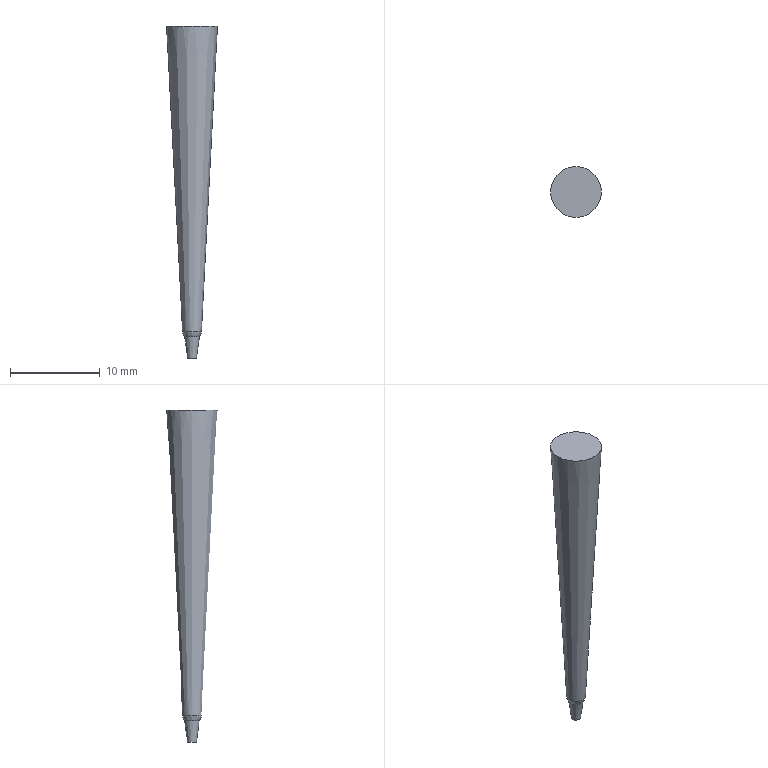Part | STEP file | SL2-MOLD_id518_xmt_txt | 1 solid | 5 faces | box 5.668 x 5.668 x 36.992 mm | volume 436.735 mm3 | plane 2 | cone 2 | spline 1
STEP:
#1=CARTESIAN_POINT('',(2.834,0.,101.));
#2=VERTEX_POINT('',#1);
#3=CARTESIAN_POINT('',(0.,0.,101.));
#4=DIRECTION('',(0.,0.,-1.));
#5=DIRECTION('',(1.,0.,0.));
#6=AXIS2_PLACEMENT_3D('',#3,#4,#5);
#7=CIRCLE('',#6,2.834);
#8=EDGE_CURVE('',#2,#2,#7,.T.);
#9=ORIENTED_EDGE('',*,*,#8,.F.);
#10=EDGE_LOOP('',(#9));
#11=FACE_OUTER_BOUND('',#10,.T.);
#12=CARTESIAN_POINT('',(1.401,-4.582,101.));
#13=DIRECTION('',(0.,0.,1.));
#14=DIRECTION('',(1.,0.,0.));
#15=AXIS2_PLACEMENT_3D('',#12,#13,#14);
#16=PLANE('',#15);
#17=ADVANCED_FACE('',(#11),#16,.T.);
#18=CARTESIAN_POINT('',(-1.05,0.,66.956));
#19=VERTEX_POINT('',#18);
#20=CARTESIAN_POINT('',(0.,0.,66.956));
#21=DIRECTION('',(0.,0.,1.));
#22=DIRECTION('',(-1.,0.,0.));
#23=AXIS2_PLACEMENT_3D('',#20,#21,#22);
#24=CIRCLE('',#23,1.05);
#25=EDGE_CURVE('',#19,#19,#24,.T.);
#26=ORIENTED_EDGE('',*,*,#25,.T.);
#27=EDGE_LOOP('',(#26));
#28=FACE_BOUND('',#27,.T.);
#29=ORIENTED_EDGE('',*,*,#8,.T.);
#30=EDGE_LOOP('',(#29));
#31=FACE_BOUND('',#30,.T.);
#32=CARTESIAN_POINT('',(0.,0.,66.008));
#33=DIRECTION('',(0.,0.,1.));
#34=DIRECTION('',(-1.,0.,0.));
#35=AXIS2_PLACEMENT_3D('',#32,#33,#34);
#36=CONICAL_SURFACE('',#35,1.,3.);
#37=ADVANCED_FACE('',(#28,#31),#36,.T.);
#38=CARTESIAN_POINT('',(0.8342,0.,66.386));
#39=VERTEX_POINT('',#38);
#40=CARTESIAN_POINT('',(0.,0.,66.386));
#41=DIRECTION('',(0.,0.,-1.));
#42=DIRECTION('',(1.,0.,0.));
#43=AXIS2_PLACEMENT_3D('',#40,#41,#42);
#44=CIRCLE('',#43,0.8342);
#45=EDGE_CURVE('',#39,#39,#44,.T.);
#46=ORIENTED_EDGE('',*,*,#45,.F.);
#47=EDGE_LOOP('',(#46));
#48=FACE_BOUND('',#47,.T.);
#49=ORIENTED_EDGE('',*,*,#25,.F.);
#50=EDGE_LOOP('',(#49));
#51=FACE_BOUND('',#50,.T.);
#52=CARTESIAN_POINT('',(-0.8342,0.,66.386));
#53=CARTESIAN_POINT('',(-0.8342,1.668,66.386));
#54=CARTESIAN_POINT('',(0.8342,1.668,66.386));
#55=CARTESIAN_POINT('',(0.8342,0.,66.386));
#56=CARTESIAN_POINT('',(0.8342,-1.668,66.386));
#57=CARTESIAN_POINT('',(-0.8342,-1.668,66.386));
#58=CARTESIAN_POINT('',(-0.8342,0.,66.386));
#59=CARTESIAN_POINT('',(-0.9645,0.,66.55));
#60=CARTESIAN_POINT('',(-0.9645,1.929,66.55));
#61=CARTESIAN_POINT('',(0.9645,1.929,66.55));
#62=CARTESIAN_POINT('',(0.9645,0.,66.55));
#63=CARTESIAN_POINT('',(0.9645,-1.929,66.55));
#64=CARTESIAN_POINT('',(-0.9645,-1.929,66.55));
#65=CARTESIAN_POINT('',(-0.9645,0.,66.55));
#66=CARTESIAN_POINT('',(-1.039,0.,66.746));
#67=CARTESIAN_POINT('',(-1.039,2.077,66.746));
#68=CARTESIAN_POINT('',(1.039,2.077,66.746));
#69=CARTESIAN_POINT('',(1.039,0.,66.746));
#70=CARTESIAN_POINT('',(1.039,-2.077,66.746));
#71=CARTESIAN_POINT('',(-1.039,-2.077,66.746));
#72=CARTESIAN_POINT('',(-1.039,0.,66.746));
#73=CARTESIAN_POINT('',(-1.05,0.,66.956));
#74=CARTESIAN_POINT('',(-1.05,2.099,66.956));
#75=CARTESIAN_POINT('',(1.05,2.099,66.956));
#76=CARTESIAN_POINT('',(1.05,0.,66.956));
#77=CARTESIAN_POINT('',(1.05,-2.099,66.956));
#78=CARTESIAN_POINT('',(-1.05,-2.099,66.956));
#79=CARTESIAN_POINT('',(-1.05,0.,66.956));
#80=(BOUNDED_SURFACE()B_SPLINE_SURFACE(3,3,((#52,#53,#54,#55,#56,#57,#58),(#59,#60,#61,#62,#63,#64,#65),(#66,#67,#68,#69,#70,#71,#72),(#73,#74,#75,#76,#77,#78,#79)),.UNSPECIFIED.,.F.,.T.,.F.)B_SPLINE_SURFACE_WITH_KNOTS((4,4),(1,3,3,3,1),(0.,1.),(-0.5,0.,0.5,1.,1.5),.UNSPECIFIED.)GEOMETRIC_REPRESENTATION_ITEM()RATIONAL_B_SPLINE_SURFACE(((1.,0.3333,0.3333,1.,0.3333,0.3333,1.),(0.9684,0.3228,0.3228,0.9684,0.3228,0.3228,0.9684),(0.9684,0.3228,0.3228,0.9684,0.3228,0.3228,0.9684),(1.,0.3333,0.3333,1.,0.3333,0.3333,1.)))REPRESENTATION_ITEM('')SURFACE());
#81=ADVANCED_FACE('',(#48,#51),#80,.T.);
#82=CARTESIAN_POINT('',(0.5,0.,64.008));
#83=VERTEX_POINT('',#82);
#84=CARTESIAN_POINT('',(0.,0.,64.008));
#85=DIRECTION('',(0.,0.,1.));
#86=DIRECTION('',(1.,0.,0.));
#87=AXIS2_PLACEMENT_3D('',#84,#85,#86);
#88=CIRCLE('',#87,0.5);
#89=EDGE_CURVE('',#83,#83,#88,.T.);
#90=ORIENTED_EDGE('',*,*,#89,.F.);
#91=EDGE_LOOP('',(#90));
#92=FACE_OUTER_BOUND('',#91,.T.);
#93=CARTESIAN_POINT('',(0.,0.,64.008));
#94=DIRECTION('',(0.,0.,-1.));
#95=DIRECTION('',(-1.,0.,0.));
#96=AXIS2_PLACEMENT_3D('',#93,#94,#95);
#97=PLANE('',#96);
#98=ADVANCED_FACE('',(#92),#97,.T.);
#99=ORIENTED_EDGE('',*,*,#45,.T.);
#100=EDGE_LOOP('',(#99));
#101=FACE_BOUND('',#100,.T.);
#102=ORIENTED_EDGE('',*,*,#89,.T.);
#103=EDGE_LOOP('',(#102));
#104=FACE_BOUND('',#103,.T.);
#105=CARTESIAN_POINT('',(0.,0.,64.008));
#106=DIRECTION('',(0.,0.,1.));
#107=DIRECTION('',(1.,0.,0.));
#108=AXIS2_PLACEMENT_3D('',#105,#106,#107);
#109=CONICAL_SURFACE('',#108,0.5,8.);
#110=ADVANCED_FACE('',(#101,#104),#109,.T.);
#111=CLOSED_SHELL('',(#17,#37,#81,#98,#110));
#112=MANIFOLD_SOLID_BREP('',#111);
#113=(LENGTH_UNIT()NAMED_UNIT(*)SI_UNIT(.MILLI.,.METRE.));
#114=UNCERTAINTY_MEASURE_WITH_UNIT(LENGTH_MEASURE(0.0254),#113,'','');
#115=(NAMED_UNIT(*)PLANE_ANGLE_UNIT()SI_UNIT($,.RADIAN.));
#116=PLANE_ANGLE_MEASURE_WITH_UNIT(PLANE_ANGLE_MEASURE(0.01745),#115);
#117=DIMENSIONAL_EXPONENTS(0.,0.,0.,0.,0.,0.,0.);
#118=(CONVERSION_BASED_UNIT('DEGREE',#116)NAMED_UNIT(#117)PLANE_ANGLE_UNIT());
#119=(NAMED_UNIT(*)SI_UNIT($,.STERADIAN.)SOLID_ANGLE_UNIT());
#120=(GEOMETRIC_REPRESENTATION_CONTEXT(3)GLOBAL_UNCERTAINTY_ASSIGNED_CONTEXT((#114))GLOBAL_UNIT_ASSIGNED_CONTEXT((#113,#118,#119))REPRESENTATION_CONTEXT('',''));
#121=ADVANCED_BREP_SHAPE_REPRESENTATION('',(#112),#120);